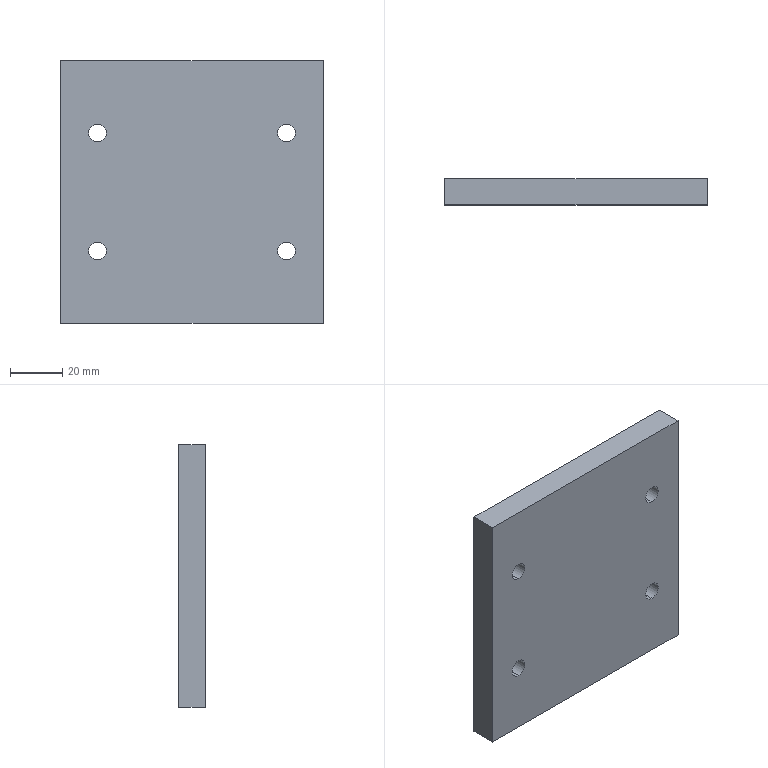Part | SolidWorks | features 3DProfileFeature 1, Extrusion 1, HoleWzd 1 | 1 solid | 14 faces | box 100 x 10 x 100 mm | volume 98547 mm3 | cylinder 8 | plane 6 | commonest cylinder face diameters 6.8 x8
STEP:
#1=CARTESIAN_POINT('',(-36.,10.,25.9));
#2=VERTEX_POINT('',#1);
#3=CARTESIAN_POINT('',(-36.,10.,19.1));
#4=VERTEX_POINT('',#3);
#5=CARTESIAN_POINT('',(-36.,10.,22.5));
#6=DIRECTION('',(0.,-1.,0.));
#7=DIRECTION('',(0.,0.,-1.));
#8=AXIS2_PLACEMENT_3D('',#5,#6,#7);
#9=CIRCLE('',#8,3.4);
#10=EDGE_CURVE('',#2,#4,#9,.T.);
#11=ORIENTED_EDGE('',*,*,#10,.F.);
#12=CARTESIAN_POINT('',(-36.,0.,25.9));
#13=VERTEX_POINT('',#12);
#14=CARTESIAN_POINT('',(-36.,0.,25.9));
#15=DIRECTION('',(0.,-1.,0.));
#16=VECTOR('',#15,1000.);
#17=LINE('',#14,#16);
#18=EDGE_CURVE('',#2,#13,#17,.T.);
#19=ORIENTED_EDGE('',*,*,#18,.T.);
#20=CARTESIAN_POINT('',(-36.,0.,19.1));
#21=VERTEX_POINT('',#20);
#22=CARTESIAN_POINT('',(-36.,0.,22.5));
#23=DIRECTION('',(0.,-1.,0.));
#24=DIRECTION('',(0.,0.,-1.));
#25=AXIS2_PLACEMENT_3D('',#22,#23,#24);
#26=CIRCLE('',#25,3.4);
#27=EDGE_CURVE('',#13,#21,#26,.T.);
#28=ORIENTED_EDGE('',*,*,#27,.T.);
#29=CARTESIAN_POINT('',(-36.,0.,19.1));
#30=DIRECTION('',(0.,-1.,0.));
#31=VECTOR('',#30,1000.);
#32=LINE('',#29,#31);
#33=EDGE_CURVE('',#4,#21,#32,.T.);
#34=ORIENTED_EDGE('',*,*,#33,.F.);
#35=EDGE_LOOP('',(#11,#19,#28,#34));
#36=FACE_OUTER_BOUND('',#35,.T.);
#37=CARTESIAN_POINT('',(-36.,0.,22.5));
#38=DIRECTION('',(0.,-1.,0.));
#39=DIRECTION('',(0.,0.,-1.));
#40=AXIS2_PLACEMENT_3D('',#37,#38,#39);
#41=CYLINDRICAL_SURFACE('',#40,3.4);
#42=ADVANCED_FACE('',(#36),#41,.F.);
#43=CARTESIAN_POINT('',(-36.,10.,-19.1));
#44=VERTEX_POINT('',#43);
#45=CARTESIAN_POINT('',(-36.,10.,-25.9));
#46=VERTEX_POINT('',#45);
#47=CARTESIAN_POINT('',(-36.,10.,-22.5));
#48=DIRECTION('',(0.,-1.,0.));
#49=DIRECTION('',(0.,0.,-1.));
#50=AXIS2_PLACEMENT_3D('',#47,#48,#49);
#51=CIRCLE('',#50,3.4);
#52=EDGE_CURVE('',#44,#46,#51,.T.);
#53=ORIENTED_EDGE('',*,*,#52,.F.);
#54=CARTESIAN_POINT('',(-36.,0.,-19.1));
#55=VERTEX_POINT('',#54);
#56=CARTESIAN_POINT('',(-36.,0.,-19.1));
#57=DIRECTION('',(0.,-1.,0.));
#58=VECTOR('',#57,1000.);
#59=LINE('',#56,#58);
#60=EDGE_CURVE('',#44,#55,#59,.T.);
#61=ORIENTED_EDGE('',*,*,#60,.T.);
#62=CARTESIAN_POINT('',(-36.,0.,-25.9));
#63=VERTEX_POINT('',#62);
#64=CARTESIAN_POINT('',(-36.,0.,-22.5));
#65=DIRECTION('',(0.,-1.,0.));
#66=DIRECTION('',(0.,0.,-1.));
#67=AXIS2_PLACEMENT_3D('',#64,#65,#66);
#68=CIRCLE('',#67,3.4);
#69=EDGE_CURVE('',#55,#63,#68,.T.);
#70=ORIENTED_EDGE('',*,*,#69,.T.);
#71=CARTESIAN_POINT('',(-36.,0.,-25.9));
#72=DIRECTION('',(0.,-1.,0.));
#73=VECTOR('',#72,1000.);
#74=LINE('',#71,#73);
#75=EDGE_CURVE('',#46,#63,#74,.T.);
#76=ORIENTED_EDGE('',*,*,#75,.F.);
#77=EDGE_LOOP('',(#53,#61,#70,#76));
#78=FACE_OUTER_BOUND('',#77,.T.);
#79=CARTESIAN_POINT('',(-36.,0.,-22.5));
#80=DIRECTION('',(0.,-1.,0.));
#81=DIRECTION('',(0.,0.,-1.));
#82=AXIS2_PLACEMENT_3D('',#79,#80,#81);
#83=CYLINDRICAL_SURFACE('',#82,3.4);
#84=ADVANCED_FACE('',(#78),#83,.F.);
#85=CARTESIAN_POINT('',(36.,10.,25.9));
#86=VERTEX_POINT('',#85);
#87=CARTESIAN_POINT('',(36.,10.,19.1));
#88=VERTEX_POINT('',#87);
#89=CARTESIAN_POINT('',(36.,10.,22.5));
#90=DIRECTION('',(0.,-1.,0.));
#91=DIRECTION('',(0.,0.,-1.));
#92=AXIS2_PLACEMENT_3D('',#89,#90,#91);
#93=CIRCLE('',#92,3.4);
#94=EDGE_CURVE('',#86,#88,#93,.T.);
#95=ORIENTED_EDGE('',*,*,#94,.F.);
#96=CARTESIAN_POINT('',(36.,0.,25.9));
#97=VERTEX_POINT('',#96);
#98=CARTESIAN_POINT('',(36.,0.,25.9));
#99=DIRECTION('',(0.,-1.,0.));
#100=VECTOR('',#99,1000.);
#101=LINE('',#98,#100);
#102=EDGE_CURVE('',#86,#97,#101,.T.);
#103=ORIENTED_EDGE('',*,*,#102,.T.);
#104=CARTESIAN_POINT('',(36.,0.,19.1));
#105=VERTEX_POINT('',#104);
#106=CARTESIAN_POINT('',(36.,0.,22.5));
#107=DIRECTION('',(0.,-1.,0.));
#108=DIRECTION('',(0.,0.,-1.));
#109=AXIS2_PLACEMENT_3D('',#106,#107,#108);
#110=CIRCLE('',#109,3.4);
#111=EDGE_CURVE('',#97,#105,#110,.T.);
#112=ORIENTED_EDGE('',*,*,#111,.T.);
#113=CARTESIAN_POINT('',(36.,0.,19.1));
#114=DIRECTION('',(0.,-1.,0.));
#115=VECTOR('',#114,1000.);
#116=LINE('',#113,#115);
#117=EDGE_CURVE('',#88,#105,#116,.T.);
#118=ORIENTED_EDGE('',*,*,#117,.F.);
#119=EDGE_LOOP('',(#95,#103,#112,#118));
#120=FACE_OUTER_BOUND('',#119,.T.);
#121=CARTESIAN_POINT('',(36.,0.,22.5));
#122=DIRECTION('',(0.,-1.,0.));
#123=DIRECTION('',(0.,0.,-1.));
#124=AXIS2_PLACEMENT_3D('',#121,#122,#123);
#125=CYLINDRICAL_SURFACE('',#124,3.4);
#126=ADVANCED_FACE('',(#120),#125,.F.);
#127=CARTESIAN_POINT('',(36.,10.,-19.1));
#128=VERTEX_POINT('',#127);
#129=CARTESIAN_POINT('',(36.,10.,-25.9));
#130=VERTEX_POINT('',#129);
#131=CARTESIAN_POINT('',(36.,10.,-22.5));
#132=DIRECTION('',(0.,-1.,0.));
#133=DIRECTION('',(0.,0.,-1.));
#134=AXIS2_PLACEMENT_3D('',#131,#132,#133);
#135=CIRCLE('',#134,3.4);
#136=EDGE_CURVE('',#128,#130,#135,.T.);
#137=ORIENTED_EDGE('',*,*,#136,.F.);
#138=CARTESIAN_POINT('',(36.,0.,-19.1));
#139=VERTEX_POINT('',#138);
#140=CARTESIAN_POINT('',(36.,0.,-19.1));
#141=DIRECTION('',(0.,-1.,0.));
#142=VECTOR('',#141,1000.);
#143=LINE('',#140,#142);
#144=EDGE_CURVE('',#128,#139,#143,.T.);
#145=ORIENTED_EDGE('',*,*,#144,.T.);
#146=CARTESIAN_POINT('',(36.,0.,-25.9));
#147=VERTEX_POINT('',#146);
#148=CARTESIAN_POINT('',(36.,0.,-22.5));
#149=DIRECTION('',(0.,-1.,0.));
#150=DIRECTION('',(0.,0.,-1.));
#151=AXIS2_PLACEMENT_3D('',#148,#149,#150);
#152=CIRCLE('',#151,3.4);
#153=EDGE_CURVE('',#139,#147,#152,.T.);
#154=ORIENTED_EDGE('',*,*,#153,.T.);
#155=CARTESIAN_POINT('',(36.,0.,-25.9));
#156=DIRECTION('',(0.,-1.,0.));
#157=VECTOR('',#156,1000.);
#158=LINE('',#155,#157);
#159=EDGE_CURVE('',#130,#147,#158,.T.);
#160=ORIENTED_EDGE('',*,*,#159,.F.);
#161=EDGE_LOOP('',(#137,#145,#154,#160));
#162=FACE_OUTER_BOUND('',#161,.T.);
#163=CARTESIAN_POINT('',(36.,0.,-22.5));
#164=DIRECTION('',(0.,-1.,0.));
#165=DIRECTION('',(0.,0.,-1.));
#166=AXIS2_PLACEMENT_3D('',#163,#164,#165);
#167=CYLINDRICAL_SURFACE('',#166,3.4);
#168=ADVANCED_FACE('',(#162),#167,.F.);
#169=CARTESIAN_POINT('',(-50.,0.,-50.));
#170=VERTEX_POINT('',#169);
#171=CARTESIAN_POINT('',(-50.,0.,50.));
#172=VERTEX_POINT('',#171);
#173=CARTESIAN_POINT('',(-50.,0.,-50.));
#174=DIRECTION('',(0.,0.,1.));
#175=VECTOR('',#174,1000.);
#176=LINE('',#173,#175);
#177=EDGE_CURVE('',#170,#172,#176,.T.);
#178=ORIENTED_EDGE('',*,*,#177,.T.);
#179=CARTESIAN_POINT('',(-50.,10.,50.));
#180=VERTEX_POINT('',#179);
#181=CARTESIAN_POINT('',(-50.,10.,50.));
#182=DIRECTION('',(0.,-1.,0.));
#183=VECTOR('',#182,1000.);
#184=LINE('',#181,#183);
#185=EDGE_CURVE('',#180,#172,#184,.T.);
#186=ORIENTED_EDGE('',*,*,#185,.F.);
#187=CARTESIAN_POINT('',(-50.,10.,-50.));
#188=VERTEX_POINT('',#187);
#189=CARTESIAN_POINT('',(-50.,10.,-50.));
#190=DIRECTION('',(0.,0.,1.));
#191=VECTOR('',#190,1000.);
#192=LINE('',#189,#191);
#193=EDGE_CURVE('',#188,#180,#192,.T.);
#194=ORIENTED_EDGE('',*,*,#193,.F.);
#195=CARTESIAN_POINT('',(-50.,10.,-50.));
#196=DIRECTION('',(0.,-1.,0.));
#197=VECTOR('',#196,1000.);
#198=LINE('',#195,#197);
#199=EDGE_CURVE('',#188,#170,#198,.T.);
#200=ORIENTED_EDGE('',*,*,#199,.T.);
#201=EDGE_LOOP('',(#178,#186,#194,#200));
#202=FACE_OUTER_BOUND('',#201,.T.);
#203=CARTESIAN_POINT('',(-50.,10.,-50.));
#204=DIRECTION('',(1.,0.,0.));
#205=DIRECTION('',(0.,0.,-1.));
#206=AXIS2_PLACEMENT_3D('',#203,#204,#205);
#207=PLANE('',#206);
#208=ADVANCED_FACE('',(#202),#207,.F.);
#209=CARTESIAN_POINT('',(50.,0.,50.));
#210=VERTEX_POINT('',#209);
#211=CARTESIAN_POINT('',(-50.,0.,50.));
#212=DIRECTION('',(1.,0.,0.));
#213=VECTOR('',#212,1000.);
#214=LINE('',#211,#213);
#215=EDGE_CURVE('',#172,#210,#214,.T.);
#216=ORIENTED_EDGE('',*,*,#215,.T.);
#217=CARTESIAN_POINT('',(50.,10.,50.));
#218=VERTEX_POINT('',#217);
#219=CARTESIAN_POINT('',(50.,10.,50.));
#220=DIRECTION('',(0.,-1.,0.));
#221=VECTOR('',#220,1000.);
#222=LINE('',#219,#221);
#223=EDGE_CURVE('',#218,#210,#222,.T.);
#224=ORIENTED_EDGE('',*,*,#223,.F.);
#225=CARTESIAN_POINT('',(-50.,10.,50.));
#226=DIRECTION('',(1.,0.,0.));
#227=VECTOR('',#226,1000.);
#228=LINE('',#225,#227);
#229=EDGE_CURVE('',#180,#218,#228,.T.);
#230=ORIENTED_EDGE('',*,*,#229,.F.);
#231=ORIENTED_EDGE('',*,*,#185,.T.);
#232=EDGE_LOOP('',(#216,#224,#230,#231));
#233=FACE_OUTER_BOUND('',#232,.T.);
#234=CARTESIAN_POINT('',(-50.,10.,50.));
#235=DIRECTION('',(0.,0.,-1.));
#236=DIRECTION('',(-1.,0.,0.));
#237=AXIS2_PLACEMENT_3D('',#234,#235,#236);
#238=PLANE('',#237);
#239=ADVANCED_FACE('',(#233),#238,.F.);
#240=CARTESIAN_POINT('',(50.,0.,-50.));
#241=VERTEX_POINT('',#240);
#242=CARTESIAN_POINT('',(50.,0.,-50.));
#243=DIRECTION('',(0.,0.,-1.));
#244=VECTOR('',#243,1000.);
#245=LINE('',#242,#244);
#246=EDGE_CURVE('',#210,#241,#245,.T.);
#247=ORIENTED_EDGE('',*,*,#246,.T.);
#248=CARTESIAN_POINT('',(50.,10.,-50.));
#249=VERTEX_POINT('',#248);
#250=CARTESIAN_POINT('',(50.,10.,-50.));
#251=DIRECTION('',(0.,-1.,0.));
#252=VECTOR('',#251,1000.);
#253=LINE('',#250,#252);
#254=EDGE_CURVE('',#249,#241,#253,.T.);
#255=ORIENTED_EDGE('',*,*,#254,.F.);
#256=CARTESIAN_POINT('',(50.,10.,-50.));
#257=DIRECTION('',(0.,0.,-1.));
#258=VECTOR('',#257,1000.);
#259=LINE('',#256,#258);
#260=EDGE_CURVE('',#218,#249,#259,.T.);
#261=ORIENTED_EDGE('',*,*,#260,.F.);
#262=ORIENTED_EDGE('',*,*,#223,.T.);
#263=EDGE_LOOP('',(#247,#255,#261,#262));
#264=FACE_OUTER_BOUND('',#263,.T.);
#265=CARTESIAN_POINT('',(50.,10.,-50.));
#266=DIRECTION('',(-1.,0.,0.));
#267=DIRECTION('',(0.,0.,1.));
#268=AXIS2_PLACEMENT_3D('',#265,#266,#267);
#269=PLANE('',#268);
#270=ADVANCED_FACE('',(#264),#269,.F.);
#271=CARTESIAN_POINT('',(-50.,0.,-50.));
#272=DIRECTION('',(-1.,0.,0.));
#273=VECTOR('',#272,1000.);
#274=LINE('',#271,#273);
#275=EDGE_CURVE('',#241,#170,#274,.T.);
#276=ORIENTED_EDGE('',*,*,#275,.T.);
#277=ORIENTED_EDGE('',*,*,#199,.F.);
#278=CARTESIAN_POINT('',(-50.,10.,-50.));
#279=DIRECTION('',(-1.,0.,0.));
#280=VECTOR('',#279,1000.);
#281=LINE('',#278,#280);
#282=EDGE_CURVE('',#249,#188,#281,.T.);
#283=ORIENTED_EDGE('',*,*,#282,.F.);
#284=ORIENTED_EDGE('',*,*,#254,.T.);
#285=EDGE_LOOP('',(#276,#277,#283,#284));
#286=FACE_OUTER_BOUND('',#285,.T.);
#287=CARTESIAN_POINT('',(-50.,10.,-50.));
#288=DIRECTION('',(0.,0.,1.));
#289=DIRECTION('',(1.,0.,0.));
#290=AXIS2_PLACEMENT_3D('',#287,#288,#289);
#291=PLANE('',#290);
#292=ADVANCED_FACE('',(#286),#291,.F.);
#293=CARTESIAN_POINT('',(-36.,10.,22.5));
#294=DIRECTION('',(0.,-1.,0.));
#295=DIRECTION('',(0.,0.,-1.));
#296=AXIS2_PLACEMENT_3D('',#293,#294,#295);
#297=CIRCLE('',#296,3.4);
#298=EDGE_CURVE('',#4,#2,#297,.T.);
#299=ORIENTED_EDGE('',*,*,#298,.T.);
#300=ORIENTED_EDGE('',*,*,#10,.T.);
#301=EDGE_LOOP('',(#299,#300));
#302=FACE_BOUND('',#301,.T.);
#303=CARTESIAN_POINT('',(-36.,10.,-22.5));
#304=DIRECTION('',(0.,-1.,0.));
#305=DIRECTION('',(0.,0.,-1.));
#306=AXIS2_PLACEMENT_3D('',#303,#304,#305);
#307=CIRCLE('',#306,3.4);
#308=EDGE_CURVE('',#46,#44,#307,.T.);
#309=ORIENTED_EDGE('',*,*,#308,.T.);
#310=ORIENTED_EDGE('',*,*,#52,.T.);
#311=EDGE_LOOP('',(#309,#310));
#312=FACE_BOUND('',#311,.T.);
#313=CARTESIAN_POINT('',(36.,10.,22.5));
#314=DIRECTION('',(0.,-1.,0.));
#315=DIRECTION('',(0.,0.,-1.));
#316=AXIS2_PLACEMENT_3D('',#313,#314,#315);
#317=CIRCLE('',#316,3.4);
#318=EDGE_CURVE('',#88,#86,#317,.T.);
#319=ORIENTED_EDGE('',*,*,#318,.T.);
#320=ORIENTED_EDGE('',*,*,#94,.T.);
#321=EDGE_LOOP('',(#319,#320));
#322=FACE_BOUND('',#321,.T.);
#323=CARTESIAN_POINT('',(36.,10.,-22.5));
#324=DIRECTION('',(0.,-1.,0.));
#325=DIRECTION('',(0.,0.,-1.));
#326=AXIS2_PLACEMENT_3D('',#323,#324,#325);
#327=CIRCLE('',#326,3.4);
#328=EDGE_CURVE('',#130,#128,#327,.T.);
#329=ORIENTED_EDGE('',*,*,#328,.T.);
#330=ORIENTED_EDGE('',*,*,#136,.T.);
#331=EDGE_LOOP('',(#329,#330));
#332=FACE_BOUND('',#331,.T.);
#333=ORIENTED_EDGE('',*,*,#193,.T.);
#334=ORIENTED_EDGE('',*,*,#229,.T.);
#335=ORIENTED_EDGE('',*,*,#260,.T.);
#336=ORIENTED_EDGE('',*,*,#282,.T.);
#337=EDGE_LOOP('',(#333,#334,#335,#336));
#338=FACE_OUTER_BOUND('',#337,.T.);
#339=CARTESIAN_POINT('',(-50.,10.,50.));
#340=DIRECTION('',(0.,1.,0.));
#341=DIRECTION('',(0.,0.,1.));
#342=AXIS2_PLACEMENT_3D('',#339,#340,#341);
#343=PLANE('',#342);
#344=ADVANCED_FACE('',(#302,#312,#322,#332,#338),#343,.T.);
#345=CARTESIAN_POINT('',(-36.,0.,22.5));
#346=DIRECTION('',(0.,-1.,0.));
#347=DIRECTION('',(0.,0.,-1.));
#348=AXIS2_PLACEMENT_3D('',#345,#346,#347);
#349=CIRCLE('',#348,3.4);
#350=EDGE_CURVE('',#21,#13,#349,.T.);
#351=ORIENTED_EDGE('',*,*,#350,.F.);
#352=ORIENTED_EDGE('',*,*,#27,.F.);
#353=EDGE_LOOP('',(#351,#352));
#354=FACE_BOUND('',#353,.T.);
#355=CARTESIAN_POINT('',(-36.,0.,-22.5));
#356=DIRECTION('',(0.,-1.,0.));
#357=DIRECTION('',(0.,0.,-1.));
#358=AXIS2_PLACEMENT_3D('',#355,#356,#357);
#359=CIRCLE('',#358,3.4);
#360=EDGE_CURVE('',#63,#55,#359,.T.);
#361=ORIENTED_EDGE('',*,*,#360,.F.);
#362=ORIENTED_EDGE('',*,*,#69,.F.);
#363=EDGE_LOOP('',(#361,#362));
#364=FACE_BOUND('',#363,.T.);
#365=CARTESIAN_POINT('',(36.,0.,22.5));
#366=DIRECTION('',(0.,-1.,0.));
#367=DIRECTION('',(0.,0.,-1.));
#368=AXIS2_PLACEMENT_3D('',#365,#366,#367);
#369=CIRCLE('',#368,3.4);
#370=EDGE_CURVE('',#105,#97,#369,.T.);
#371=ORIENTED_EDGE('',*,*,#370,.F.);
#372=ORIENTED_EDGE('',*,*,#111,.F.);
#373=EDGE_LOOP('',(#371,#372));
#374=FACE_BOUND('',#373,.T.);
#375=CARTESIAN_POINT('',(36.,0.,-22.5));
#376=DIRECTION('',(0.,-1.,0.));
#377=DIRECTION('',(0.,0.,-1.));
#378=AXIS2_PLACEMENT_3D('',#375,#376,#377);
#379=CIRCLE('',#378,3.4);
#380=EDGE_CURVE('',#147,#139,#379,.T.);
#381=ORIENTED_EDGE('',*,*,#380,.F.);
#382=ORIENTED_EDGE('',*,*,#153,.F.);
#383=EDGE_LOOP('',(#381,#382));
#384=FACE_BOUND('',#383,.T.);
#385=ORIENTED_EDGE('',*,*,#177,.F.);
#386=ORIENTED_EDGE('',*,*,#275,.F.);
#387=ORIENTED_EDGE('',*,*,#246,.F.);
#388=ORIENTED_EDGE('',*,*,#215,.F.);
#389=EDGE_LOOP('',(#385,#386,#387,#388));
#390=FACE_OUTER_BOUND('',#389,.T.);
#391=CARTESIAN_POINT('',(-50.,0.,50.));
#392=DIRECTION('',(0.,1.,0.));
#393=DIRECTION('',(0.,0.,1.));
#394=AXIS2_PLACEMENT_3D('',#391,#392,#393);
#395=PLANE('',#394);
#396=ADVANCED_FACE('',(#354,#364,#374,#384,#390),#395,.F.);
#397=ORIENTED_EDGE('',*,*,#144,.F.);
#398=ORIENTED_EDGE('',*,*,#328,.F.);
#399=ORIENTED_EDGE('',*,*,#159,.T.);
#400=ORIENTED_EDGE('',*,*,#380,.T.);
#401=EDGE_LOOP('',(#397,#398,#399,#400));
#402=FACE_OUTER_BOUND('',#401,.T.);
#403=CARTESIAN_POINT('',(36.,0.,-22.5));
#404=DIRECTION('',(0.,-1.,0.));
#405=DIRECTION('',(0.,0.,-1.));
#406=AXIS2_PLACEMENT_3D('',#403,#404,#405);
#407=CYLINDRICAL_SURFACE('',#406,3.4);
#408=ADVANCED_FACE('',(#402),#407,.F.);
#409=ORIENTED_EDGE('',*,*,#102,.F.);
#410=ORIENTED_EDGE('',*,*,#318,.F.);
#411=ORIENTED_EDGE('',*,*,#117,.T.);
#412=ORIENTED_EDGE('',*,*,#370,.T.);
#413=EDGE_LOOP('',(#409,#410,#411,#412));
#414=FACE_OUTER_BOUND('',#413,.T.);
#415=CARTESIAN_POINT('',(36.,0.,22.5));
#416=DIRECTION('',(0.,-1.,0.));
#417=DIRECTION('',(0.,0.,-1.));
#418=AXIS2_PLACEMENT_3D('',#415,#416,#417);
#419=CYLINDRICAL_SURFACE('',#418,3.4);
#420=ADVANCED_FACE('',(#414),#419,.F.);
#421=ORIENTED_EDGE('',*,*,#60,.F.);
#422=ORIENTED_EDGE('',*,*,#308,.F.);
#423=ORIENTED_EDGE('',*,*,#75,.T.);
#424=ORIENTED_EDGE('',*,*,#360,.T.);
#425=EDGE_LOOP('',(#421,#422,#423,#424));
#426=FACE_OUTER_BOUND('',#425,.T.);
#427=CARTESIAN_POINT('',(-36.,0.,-22.5));
#428=DIRECTION('',(0.,-1.,0.));
#429=DIRECTION('',(0.,0.,-1.));
#430=AXIS2_PLACEMENT_3D('',#427,#428,#429);
#431=CYLINDRICAL_SURFACE('',#430,3.4);
#432=ADVANCED_FACE('',(#426),#431,.F.);
#433=ORIENTED_EDGE('',*,*,#18,.F.);
#434=ORIENTED_EDGE('',*,*,#298,.F.);
#435=ORIENTED_EDGE('',*,*,#33,.T.);
#436=ORIENTED_EDGE('',*,*,#350,.T.);
#437=EDGE_LOOP('',(#433,#434,#435,#436));
#438=FACE_OUTER_BOUND('',#437,.T.);
#439=CARTESIAN_POINT('',(-36.,0.,22.5));
#440=DIRECTION('',(0.,-1.,0.));
#441=DIRECTION('',(0.,0.,-1.));
#442=AXIS2_PLACEMENT_3D('',#439,#440,#441);
#443=CYLINDRICAL_SURFACE('',#442,3.4);
#444=ADVANCED_FACE('',(#438),#443,.F.);
#445=CLOSED_SHELL('',(#42,#84,#126,#168,#208,#239,#270,#292,#344,#396,#408,#420,#432,#444));
#446=MANIFOLD_SOLID_BREP('',#445);
#447=CARTESIAN_POINT('',(0.,0.,0.));
#448=DIRECTION('',(0.,0.,1.));
#449=DIRECTION('',(1.,0.,0.));
#450=AXIS2_PLACEMENT_3D('',#447,#448,#449);
#451=(LENGTH_UNIT()NAMED_UNIT(*)SI_UNIT(.MILLI.,.METRE.));
#452=UNCERTAINTY_MEASURE_WITH_UNIT(LENGTH_MEASURE(0.00001),#451,'','');
#453=(NAMED_UNIT(*)PLANE_ANGLE_UNIT()SI_UNIT($,.RADIAN.));
#454=(NAMED_UNIT(*)SI_UNIT($,.STERADIAN.)SOLID_ANGLE_UNIT());
#455=(GEOMETRIC_REPRESENTATION_CONTEXT(3)GLOBAL_UNCERTAINTY_ASSIGNED_CONTEXT((#452))GLOBAL_UNIT_ASSIGNED_CONTEXT((#451,#453,#454))REPRESENTATION_CONTEXT('',''));
#456=ADVANCED_BREP_SHAPE_REPRESENTATION('',(#446,#450),#455);